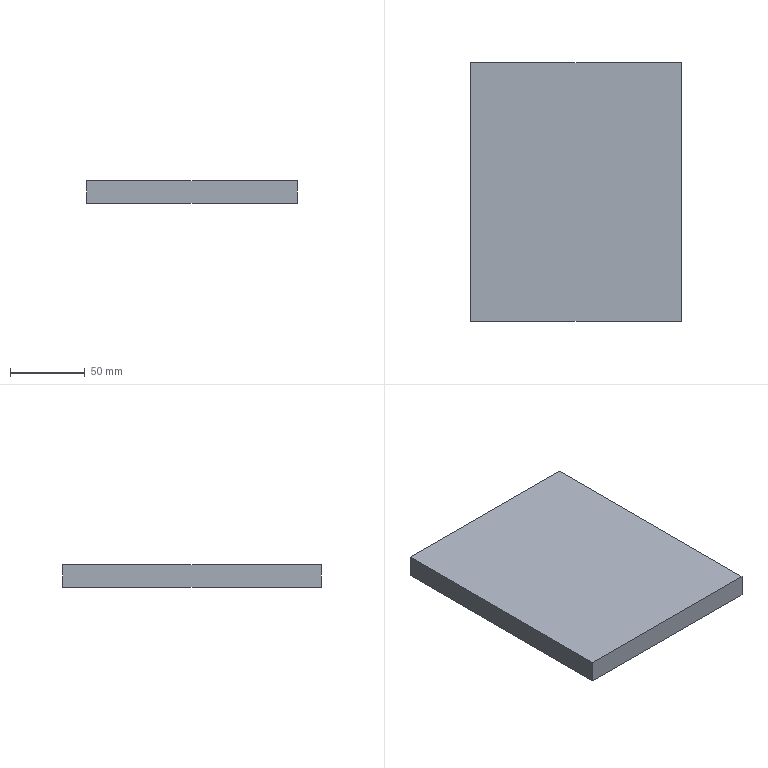Part | STEP file | 1 solid | 6 faces | box 140.887 x 173 x 15 mm | volume 365603 mm3 | plane 6
STEP:
#1=CARTESIAN_POINT('',(0.,0.,0.));
#2=DIRECTION('',(0.,0.,1.));
#3=DIRECTION('',(1.,0.,0.));
#4=AXIS2_PLACEMENT_3D('',#1,#2,#3);
#5=CARTESIAN_POINT('',(270.205,527.014,181.115));
#6=VERTEX_POINT('',#5);
#7=CARTESIAN_POINT('',(270.205,354.014,181.115));
#8=VERTEX_POINT('',#7);
#9=CARTESIAN_POINT('',(270.205,527.014,181.115));
#10=DIRECTION('',(0.,-1.,0.));
#11=VECTOR('',#10,1.);
#12=LINE('',#9,#11);
#13=CARTESIAN_POINT('',(270.205,527.014,196.115));
#14=DIRECTION('',(1.,0.,0.));
#15=DIRECTION('',(0.,0.,-1.));
#16=AXIS2_PLACEMENT_3D('',#13,#14,#15);
#17=PLANE('',#16);
#18=CARTESIAN_POINT('',(15.,0.));
#19=DIRECTION('',(0.,-1.));
#20=VECTOR('',#19,1.);
#21=LINE('',#18,#20);
#22=(GEOMETRIC_REPRESENTATION_CONTEXT(2)PARAMETRIC_REPRESENTATION_CONTEXT()REPRESENTATION_CONTEXT('',''));
#23=DEFINITIONAL_REPRESENTATION('',(#21),#22);
#24=PCURVE('',#17,#23);
#25=CARTESIAN_POINT('',(0.,0.,181.115));
#26=DIRECTION('',(0.,0.,1.));
#27=DIRECTION('',(1.,0.,0.));
#28=AXIS2_PLACEMENT_3D('',#25,#26,#27);
#29=PLANE('',#28);
#30=CARTESIAN_POINT('',(270.205,527.014));
#31=DIRECTION('',(0.,-1.));
#32=VECTOR('',#31,1.);
#33=LINE('',#30,#32);
#34=(GEOMETRIC_REPRESENTATION_CONTEXT(2)PARAMETRIC_REPRESENTATION_CONTEXT()REPRESENTATION_CONTEXT('',''));
#35=DEFINITIONAL_REPRESENTATION('',(#33),#34);
#36=PCURVE('',#29,#35);
#37=SURFACE_CURVE('',#12,(#24,#36),.PCURVE_S1.);
#38=EDGE_CURVE('',#6,#8,#37,.T.);
#39=ORIENTED_EDGE('',*,*,#38,.T.);
#40=CARTESIAN_POINT('',(270.205,354.014,196.115));
#41=VERTEX_POINT('',#40);
#42=CARTESIAN_POINT('',(270.205,354.014,196.115));
#43=DIRECTION('',(0.,0.,-1.));
#44=VECTOR('',#43,1.);
#45=LINE('',#42,#44);
#46=CARTESIAN_POINT('',(0.,-173.));
#47=DIRECTION('',(1.,0.));
#48=VECTOR('',#47,1.);
#49=LINE('',#46,#48);
#50=(GEOMETRIC_REPRESENTATION_CONTEXT(2)PARAMETRIC_REPRESENTATION_CONTEXT()REPRESENTATION_CONTEXT('',''));
#51=DEFINITIONAL_REPRESENTATION('',(#49),#50);
#52=PCURVE('',#17,#51);
#53=CARTESIAN_POINT('',(270.205,354.014,196.115));
#54=DIRECTION('',(0.,1.,0.));
#55=DIRECTION('',(0.,0.,1.));
#56=AXIS2_PLACEMENT_3D('',#53,#54,#55);
#57=PLANE('',#56);
#58=CARTESIAN_POINT('',(0.,0.));
#59=DIRECTION('',(-1.,0.));
#60=VECTOR('',#59,1.);
#61=LINE('',#58,#60);
#62=(GEOMETRIC_REPRESENTATION_CONTEXT(2)PARAMETRIC_REPRESENTATION_CONTEXT()REPRESENTATION_CONTEXT('',''));
#63=DEFINITIONAL_REPRESENTATION('',(#61),#62);
#64=PCURVE('',#57,#63);
#65=SURFACE_CURVE('',#45,(#52,#64),.PCURVE_S1.);
#66=EDGE_CURVE('',#41,#8,#65,.T.);
#67=ORIENTED_EDGE('',*,*,#66,.F.);
#68=CARTESIAN_POINT('',(270.205,527.014,196.115));
#69=VERTEX_POINT('',#68);
#70=CARTESIAN_POINT('',(270.205,527.014,196.115));
#71=DIRECTION('',(0.,-1.,0.));
#72=VECTOR('',#71,1.);
#73=LINE('',#70,#72);
#74=CARTESIAN_POINT('',(0.,0.));
#75=DIRECTION('',(0.,-1.));
#76=VECTOR('',#75,1.);
#77=LINE('',#74,#76);
#78=(GEOMETRIC_REPRESENTATION_CONTEXT(2)PARAMETRIC_REPRESENTATION_CONTEXT()REPRESENTATION_CONTEXT('',''));
#79=DEFINITIONAL_REPRESENTATION('',(#77),#78);
#80=PCURVE('',#17,#79);
#81=CARTESIAN_POINT('',(0.,0.,196.115));
#82=DIRECTION('',(0.,0.,1.));
#83=DIRECTION('',(1.,0.,0.));
#84=AXIS2_PLACEMENT_3D('',#81,#82,#83);
#85=PLANE('',#84);
#86=CARTESIAN_POINT('',(270.205,527.014));
#87=DIRECTION('',(0.,-1.));
#88=VECTOR('',#87,1.);
#89=LINE('',#86,#88);
#90=(GEOMETRIC_REPRESENTATION_CONTEXT(2)PARAMETRIC_REPRESENTATION_CONTEXT()REPRESENTATION_CONTEXT('',''));
#91=DEFINITIONAL_REPRESENTATION('',(#89),#90);
#92=PCURVE('',#85,#91);
#93=SURFACE_CURVE('',#73,(#80,#92),.PCURVE_S1.);
#94=EDGE_CURVE('',#69,#41,#93,.T.);
#95=ORIENTED_EDGE('',*,*,#94,.F.);
#96=CARTESIAN_POINT('',(270.205,527.014,196.115));
#97=DIRECTION('',(0.,0.,-1.));
#98=VECTOR('',#97,1.);
#99=LINE('',#96,#98);
#100=CARTESIAN_POINT('',(0.,0.));
#101=DIRECTION('',(1.,0.));
#102=VECTOR('',#101,1.);
#103=LINE('',#100,#102);
#104=(GEOMETRIC_REPRESENTATION_CONTEXT(2)PARAMETRIC_REPRESENTATION_CONTEXT()REPRESENTATION_CONTEXT('',''));
#105=DEFINITIONAL_REPRESENTATION('',(#103),#104);
#106=PCURVE('',#17,#105);
#107=CARTESIAN_POINT('',(270.205,527.014,196.115));
#108=DIRECTION('',(0.,-1.,0.));
#109=DIRECTION('',(0.,0.,-1.));
#110=AXIS2_PLACEMENT_3D('',#107,#108,#109);
#111=PLANE('',#110);
#112=CARTESIAN_POINT('',(0.,0.));
#113=DIRECTION('',(1.,0.));
#114=VECTOR('',#113,1.);
#115=LINE('',#112,#114);
#116=(GEOMETRIC_REPRESENTATION_CONTEXT(2)PARAMETRIC_REPRESENTATION_CONTEXT()REPRESENTATION_CONTEXT('',''));
#117=DEFINITIONAL_REPRESENTATION('',(#115),#116);
#118=PCURVE('',#111,#117);
#119=SURFACE_CURVE('',#99,(#106,#118),.PCURVE_S1.);
#120=EDGE_CURVE('',#69,#6,#119,.T.);
#121=ORIENTED_EDGE('',*,*,#120,.T.);
#122=EDGE_LOOP('',(#39,#67,#95,#121));
#123=FACE_BOUND('',#122,.T.);
#124=ADVANCED_FACE('',(#123),#17,.F.);
#125=CARTESIAN_POINT('',(411.092,354.014,181.115));
#126=VERTEX_POINT('',#125);
#127=CARTESIAN_POINT('',(270.205,354.014,181.115));
#128=DIRECTION('',(1.,0.,0.));
#129=VECTOR('',#128,1.);
#130=LINE('',#127,#129);
#131=CARTESIAN_POINT('',(-15.,0.));
#132=DIRECTION('',(0.,1.));
#133=VECTOR('',#132,1.);
#134=LINE('',#131,#133);
#135=(GEOMETRIC_REPRESENTATION_CONTEXT(2)PARAMETRIC_REPRESENTATION_CONTEXT()REPRESENTATION_CONTEXT('',''));
#136=DEFINITIONAL_REPRESENTATION('',(#134),#135);
#137=PCURVE('',#57,#136);
#138=CARTESIAN_POINT('',(270.205,354.014));
#139=DIRECTION('',(1.,0.));
#140=VECTOR('',#139,1.);
#141=LINE('',#138,#140);
#142=(GEOMETRIC_REPRESENTATION_CONTEXT(2)PARAMETRIC_REPRESENTATION_CONTEXT()REPRESENTATION_CONTEXT('',''));
#143=DEFINITIONAL_REPRESENTATION('',(#141),#142);
#144=PCURVE('',#29,#143);
#145=SURFACE_CURVE('',#130,(#137,#144),.PCURVE_S1.);
#146=EDGE_CURVE('',#8,#126,#145,.T.);
#147=ORIENTED_EDGE('',*,*,#146,.T.);
#148=CARTESIAN_POINT('',(411.092,354.014,196.115));
#149=VERTEX_POINT('',#148);
#150=CARTESIAN_POINT('',(411.092,354.014,196.115));
#151=DIRECTION('',(0.,0.,-1.));
#152=VECTOR('',#151,1.);
#153=LINE('',#150,#152);
#154=CARTESIAN_POINT('',(0.,140.887));
#155=DIRECTION('',(-1.,0.));
#156=VECTOR('',#155,1.);
#157=LINE('',#154,#156);
#158=(GEOMETRIC_REPRESENTATION_CONTEXT(2)PARAMETRIC_REPRESENTATION_CONTEXT()REPRESENTATION_CONTEXT('',''));
#159=DEFINITIONAL_REPRESENTATION('',(#157),#158);
#160=PCURVE('',#57,#159);
#161=CARTESIAN_POINT('',(411.092,527.014,196.115));
#162=DIRECTION('',(-1.,0.,0.));
#163=DIRECTION('',(0.,0.,1.));
#164=AXIS2_PLACEMENT_3D('',#161,#162,#163);
#165=PLANE('',#164);
#166=CARTESIAN_POINT('',(0.,-173.));
#167=DIRECTION('',(-1.,0.));
#168=VECTOR('',#167,1.);
#169=LINE('',#166,#168);
#170=(GEOMETRIC_REPRESENTATION_CONTEXT(2)PARAMETRIC_REPRESENTATION_CONTEXT()REPRESENTATION_CONTEXT('',''));
#171=DEFINITIONAL_REPRESENTATION('',(#169),#170);
#172=PCURVE('',#165,#171);
#173=SURFACE_CURVE('',#153,(#160,#172),.PCURVE_S1.);
#174=EDGE_CURVE('',#149,#126,#173,.T.);
#175=ORIENTED_EDGE('',*,*,#174,.F.);
#176=CARTESIAN_POINT('',(270.205,354.014,196.115));
#177=DIRECTION('',(1.,0.,0.));
#178=VECTOR('',#177,1.);
#179=LINE('',#176,#178);
#180=CARTESIAN_POINT('',(0.,0.));
#181=DIRECTION('',(0.,1.));
#182=VECTOR('',#181,1.);
#183=LINE('',#180,#182);
#184=(GEOMETRIC_REPRESENTATION_CONTEXT(2)PARAMETRIC_REPRESENTATION_CONTEXT()REPRESENTATION_CONTEXT('',''));
#185=DEFINITIONAL_REPRESENTATION('',(#183),#184);
#186=PCURVE('',#57,#185);
#187=CARTESIAN_POINT('',(270.205,354.014));
#188=DIRECTION('',(1.,0.));
#189=VECTOR('',#188,1.);
#190=LINE('',#187,#189);
#191=(GEOMETRIC_REPRESENTATION_CONTEXT(2)PARAMETRIC_REPRESENTATION_CONTEXT()REPRESENTATION_CONTEXT('',''));
#192=DEFINITIONAL_REPRESENTATION('',(#190),#191);
#193=PCURVE('',#85,#192);
#194=SURFACE_CURVE('',#179,(#186,#193),.PCURVE_S1.);
#195=EDGE_CURVE('',#41,#149,#194,.T.);
#196=ORIENTED_EDGE('',*,*,#195,.F.);
#197=ORIENTED_EDGE('',*,*,#66,.T.);
#198=EDGE_LOOP('',(#147,#175,#196,#197));
#199=FACE_BOUND('',#198,.T.);
#200=ADVANCED_FACE('',(#199),#57,.F.);
#201=CARTESIAN_POINT('',(411.092,527.014,181.115));
#202=VERTEX_POINT('',#201);
#203=CARTESIAN_POINT('',(411.092,527.014,181.115));
#204=DIRECTION('',(0.,1.,0.));
#205=VECTOR('',#204,1.);
#206=LINE('',#203,#205);
#207=CARTESIAN_POINT('',(-15.,0.));
#208=DIRECTION('',(0.,1.));
#209=VECTOR('',#208,1.);
#210=LINE('',#207,#209);
#211=(GEOMETRIC_REPRESENTATION_CONTEXT(2)PARAMETRIC_REPRESENTATION_CONTEXT()REPRESENTATION_CONTEXT('',''));
#212=DEFINITIONAL_REPRESENTATION('',(#210),#211);
#213=PCURVE('',#165,#212);
#214=CARTESIAN_POINT('',(411.092,527.014));
#215=DIRECTION('',(0.,1.));
#216=VECTOR('',#215,1.);
#217=LINE('',#214,#216);
#218=(GEOMETRIC_REPRESENTATION_CONTEXT(2)PARAMETRIC_REPRESENTATION_CONTEXT()REPRESENTATION_CONTEXT('',''));
#219=DEFINITIONAL_REPRESENTATION('',(#217),#218);
#220=PCURVE('',#29,#219);
#221=SURFACE_CURVE('',#206,(#213,#220),.PCURVE_S1.);
#222=EDGE_CURVE('',#126,#202,#221,.T.);
#223=ORIENTED_EDGE('',*,*,#222,.T.);
#224=CARTESIAN_POINT('',(411.092,527.014,196.115));
#225=VERTEX_POINT('',#224);
#226=CARTESIAN_POINT('',(411.092,527.014,196.115));
#227=DIRECTION('',(0.,0.,-1.));
#228=VECTOR('',#227,1.);
#229=LINE('',#226,#228);
#230=CARTESIAN_POINT('',(0.,0.));
#231=DIRECTION('',(-1.,0.));
#232=VECTOR('',#231,1.);
#233=LINE('',#230,#232);
#234=(GEOMETRIC_REPRESENTATION_CONTEXT(2)PARAMETRIC_REPRESENTATION_CONTEXT()REPRESENTATION_CONTEXT('',''));
#235=DEFINITIONAL_REPRESENTATION('',(#233),#234);
#236=PCURVE('',#165,#235);
#237=CARTESIAN_POINT('',(0.,140.887));
#238=DIRECTION('',(1.,0.));
#239=VECTOR('',#238,1.);
#240=LINE('',#237,#239);
#241=(GEOMETRIC_REPRESENTATION_CONTEXT(2)PARAMETRIC_REPRESENTATION_CONTEXT()REPRESENTATION_CONTEXT('',''));
#242=DEFINITIONAL_REPRESENTATION('',(#240),#241);
#243=PCURVE('',#111,#242);
#244=SURFACE_CURVE('',#229,(#236,#243),.PCURVE_S1.);
#245=EDGE_CURVE('',#225,#202,#244,.T.);
#246=ORIENTED_EDGE('',*,*,#245,.F.);
#247=CARTESIAN_POINT('',(411.092,527.014,196.115));
#248=DIRECTION('',(0.,1.,0.));
#249=VECTOR('',#248,1.);
#250=LINE('',#247,#249);
#251=CARTESIAN_POINT('',(0.,0.));
#252=DIRECTION('',(0.,1.));
#253=VECTOR('',#252,1.);
#254=LINE('',#251,#253);
#255=(GEOMETRIC_REPRESENTATION_CONTEXT(2)PARAMETRIC_REPRESENTATION_CONTEXT()REPRESENTATION_CONTEXT('',''));
#256=DEFINITIONAL_REPRESENTATION('',(#254),#255);
#257=PCURVE('',#165,#256);
#258=CARTESIAN_POINT('',(411.092,527.014));
#259=DIRECTION('',(0.,1.));
#260=VECTOR('',#259,1.);
#261=LINE('',#258,#260);
#262=(GEOMETRIC_REPRESENTATION_CONTEXT(2)PARAMETRIC_REPRESENTATION_CONTEXT()REPRESENTATION_CONTEXT('',''));
#263=DEFINITIONAL_REPRESENTATION('',(#261),#262);
#264=PCURVE('',#85,#263);
#265=SURFACE_CURVE('',#250,(#257,#264),.PCURVE_S1.);
#266=EDGE_CURVE('',#149,#225,#265,.T.);
#267=ORIENTED_EDGE('',*,*,#266,.F.);
#268=ORIENTED_EDGE('',*,*,#174,.T.);
#269=EDGE_LOOP('',(#223,#246,#267,#268));
#270=FACE_BOUND('',#269,.T.);
#271=ADVANCED_FACE('',(#270),#165,.F.);
#272=CARTESIAN_POINT('',(270.205,527.014,181.115));
#273=DIRECTION('',(-1.,0.,0.));
#274=VECTOR('',#273,1.);
#275=LINE('',#272,#274);
#276=CARTESIAN_POINT('',(15.,0.));
#277=DIRECTION('',(0.,-1.));
#278=VECTOR('',#277,1.);
#279=LINE('',#276,#278);
#280=(GEOMETRIC_REPRESENTATION_CONTEXT(2)PARAMETRIC_REPRESENTATION_CONTEXT()REPRESENTATION_CONTEXT('',''));
#281=DEFINITIONAL_REPRESENTATION('',(#279),#280);
#282=PCURVE('',#111,#281);
#283=CARTESIAN_POINT('',(270.205,527.014));
#284=DIRECTION('',(-1.,0.));
#285=VECTOR('',#284,1.);
#286=LINE('',#283,#285);
#287=(GEOMETRIC_REPRESENTATION_CONTEXT(2)PARAMETRIC_REPRESENTATION_CONTEXT()REPRESENTATION_CONTEXT('',''));
#288=DEFINITIONAL_REPRESENTATION('',(#286),#287);
#289=PCURVE('',#29,#288);
#290=SURFACE_CURVE('',#275,(#282,#289),.PCURVE_S1.);
#291=EDGE_CURVE('',#202,#6,#290,.T.);
#292=ORIENTED_EDGE('',*,*,#291,.T.);
#293=ORIENTED_EDGE('',*,*,#120,.F.);
#294=CARTESIAN_POINT('',(270.205,527.014,196.115));
#295=DIRECTION('',(-1.,0.,0.));
#296=VECTOR('',#295,1.);
#297=LINE('',#294,#296);
#298=CARTESIAN_POINT('',(0.,0.));
#299=DIRECTION('',(0.,-1.));
#300=VECTOR('',#299,1.);
#301=LINE('',#298,#300);
#302=(GEOMETRIC_REPRESENTATION_CONTEXT(2)PARAMETRIC_REPRESENTATION_CONTEXT()REPRESENTATION_CONTEXT('',''));
#303=DEFINITIONAL_REPRESENTATION('',(#301),#302);
#304=PCURVE('',#111,#303);
#305=CARTESIAN_POINT('',(270.205,527.014));
#306=DIRECTION('',(-1.,0.));
#307=VECTOR('',#306,1.);
#308=LINE('',#305,#307);
#309=(GEOMETRIC_REPRESENTATION_CONTEXT(2)PARAMETRIC_REPRESENTATION_CONTEXT()REPRESENTATION_CONTEXT('',''));
#310=DEFINITIONAL_REPRESENTATION('',(#308),#309);
#311=PCURVE('',#85,#310);
#312=SURFACE_CURVE('',#297,(#304,#311),.PCURVE_S1.);
#313=EDGE_CURVE('',#225,#69,#312,.T.);
#314=ORIENTED_EDGE('',*,*,#313,.F.);
#315=ORIENTED_EDGE('',*,*,#245,.T.);
#316=EDGE_LOOP('',(#292,#293,#314,#315));
#317=FACE_BOUND('',#316,.T.);
#318=ADVANCED_FACE('',(#317),#111,.F.);
#319=ORIENTED_EDGE('',*,*,#94,.T.);
#320=ORIENTED_EDGE('',*,*,#195,.T.);
#321=ORIENTED_EDGE('',*,*,#266,.T.);
#322=ORIENTED_EDGE('',*,*,#313,.T.);
#323=EDGE_LOOP('',(#319,#320,#321,#322));
#324=FACE_BOUND('',#323,.T.);
#325=ADVANCED_FACE('',(#324),#85,.T.);
#326=ORIENTED_EDGE('',*,*,#38,.F.);
#327=ORIENTED_EDGE('',*,*,#291,.F.);
#328=ORIENTED_EDGE('',*,*,#222,.F.);
#329=ORIENTED_EDGE('',*,*,#146,.F.);
#330=EDGE_LOOP('',(#326,#327,#328,#329));
#331=FACE_BOUND('',#330,.T.);
#332=ADVANCED_FACE('',(#331),#29,.F.);
#333=CLOSED_SHELL('',(#124,#200,#271,#318,#325,#332));
#334=MANIFOLD_SOLID_BREP('',#333);
#335=(LENGTH_UNIT()NAMED_UNIT(*)SI_UNIT(.MILLI.,.METRE.));
#336=UNCERTAINTY_MEASURE_WITH_UNIT(LENGTH_MEASURE(0.0000001),#335,'','');
#337=(NAMED_UNIT(*)PLANE_ANGLE_UNIT()SI_UNIT($,.RADIAN.));
#338=(NAMED_UNIT(*)SI_UNIT($,.STERADIAN.)SOLID_ANGLE_UNIT());
#339=(GEOMETRIC_REPRESENTATION_CONTEXT(3)GLOBAL_UNCERTAINTY_ASSIGNED_CONTEXT((#336))GLOBAL_UNIT_ASSIGNED_CONTEXT((#335,#337,#338))REPRESENTATION_CONTEXT('',''));
#340=ADVANCED_BREP_SHAPE_REPRESENTATION('',(#4,#334),#339);